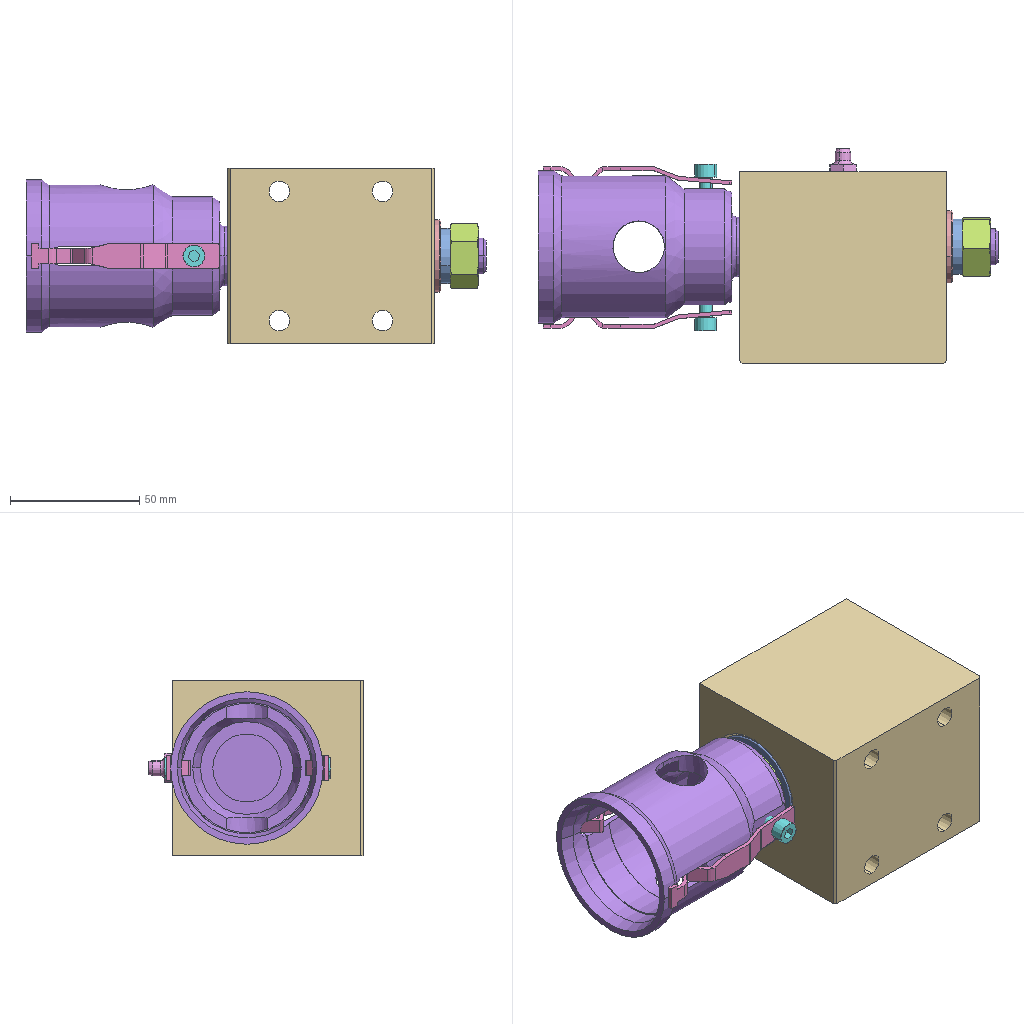Assembly | SolidWorks | 10 different items | 13 placed | box 178 x 83 x 68 mm
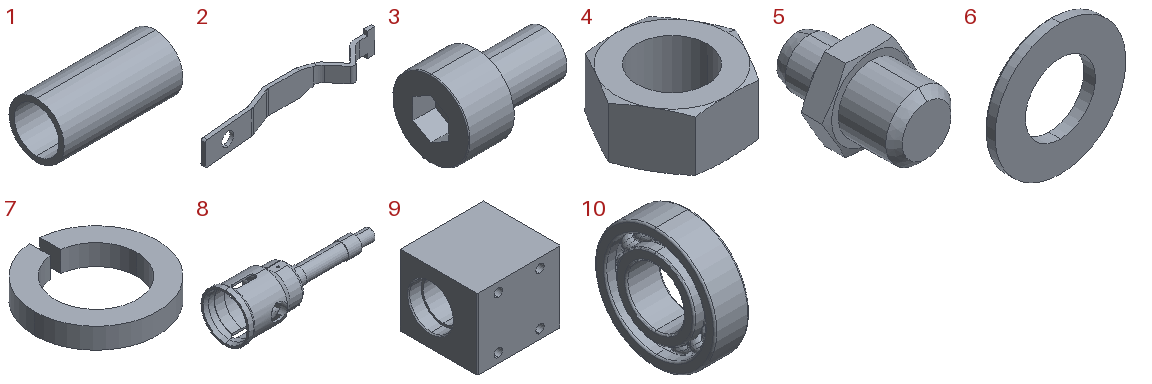Parts list (item | quantity | size | volume | features):
1 | x1 | 56 x 26 x 26 mm | 10336 mm3 | features Extrusion 1
2 | x2 | 73 x 9 x 9.5 mm | 954.396 mm3 | features Extrusion 1, ICE 1
3 | x2 | 13 x 8.5 x 8.5 mm | 404.848 mm3 | features BlendCut 1, Cut 1, Fillet 1, LPattern 1, RevCut 1, Revolution 1
4 | x1 | 25.4 x 21.997 x 11 mm | 2905 mm3 | features Cut 2, Chamfer 1, Extrusion 1
5 | x1 | 11.547 x 15.8 x 10 mm | 760.457 mm3 | features RevCut 2, Chamfer 1, Extrusion 1, ICE 1, Revolution 1
6 | x1 | 28 x 2.5 x 28 mm | 1081 mm3 | features Revolution 1
7 | x1 | 21.361 x 21.323 x 3.6 mm | 696.819 mm3 | features Extrusion 1
8 | x1 | 178 x 59 x 59 mm | 74305 mm3 | features ICE 3, MirrorPattern 1, Revolution 1
9 | x1 | 80 x 74 x 68 mm | 288342 mm3 | features MirrorPattern 3, Chamfer 2, HoleWzd 2, ICE 2, Extrusion 1, MirrorSolid 1
10 | x2 | 12 x 42 x 42 mm | 9401 mm3 | features Revolution 4, CirPattern 2, RefAxis 1, RevCut 1
Mates (type | each side: item.copy, entity, surface, feature):
Concentric | 10.1 face cylinder Revolve1 | 9.1 face cylinder Mirror3
Coincident | 10.1 face plane Revolve1 | 9.1 face plane Mirror2
Coincident | 10.2 face plane Revolve1 | 9.1 face plane Boss-Extrude1
Concentric | 10.2 face cylinder Revolve1 | 9.1 face cylinder Cut-Extrude4
Concentric | 10.1 face cylinder Revolve1 | 8.1 face cylinder Revolve1
Coincident | 10.1 face plane Revolve1 | 8.1 face plane Revolve1
Concentric | 3.1 face cylinder Base-Revolve | 8.1 face cylinder Cut-Extrude1
DistanceDim | 2.1 face plane Boss-Extrude1 | 8.1 face cylinder Revolve1
Parallel | 2.1 face plane Boss-Extrude1 | 8.1 face plane Mirror1
DistanceDim | 3.1 face plane Base-Revolve | 8.1 face plane Mirror1
Concentric | 3.2 face cylinder Base-Revolve | 8.1 face cylinder Cut-Extrude1
DistanceDim | 8.1 face plane Cut-Extrude2 | 3.2 face plane Base-Revolve
Parallel | 2.2 face plane Boss-Extrude1 | 8.1 face plane Cut-Extrude2
DistanceDim | 2.2 face plane Boss-Extrude1 | 8.1 face cylinder Revolve1
Concentric | 2.2 face cylinder Cut-Extrude1 | 3.2 face cylinder Base-Revolve
Concentric | 2.1 face cylinder Cut-Extrude1 | 3.1 face cylinder Base-Revolve
Concentric | 8.1 face cylinder Revolve1 | 1.1 face cylinder Boss-Extrude1
Coincident | 10.1 face plane Revolve1 | 1.1 face plane Boss-Extrude1
Coincident | 9.1 face plane Boss-Extrude1 | 6.1 face plane Base-Revolve
Concentric | 8.1 face cylinder Revolve1 | 6.1 face cylinder Base-Revolve
Concentric | 8.1 face cylinder Revolve1 | 7.1 face cylinder Extrude1
Coincident | 6.1 face plane Base-Revolve | 7.1 face plane Extrude1
Concentric | 8.1 face cylinder Revolve1 | 4.1 face cylinder Base-Extrude
Coincident | 7.1 face plane Extrude1 | 4.1 face plane Base-Extrude
Width | 9.1 face plane Boss-Extrude1 | 9.1 face plane Boss-Extrude1 | 2.1 face plane Boss-Extrude1 | 2.1 face plane Boss-Extrude1
Concentric | 9.1 face cylinder M8 Tapped Hole1 | 5.1 face cylinder Boss-Extrude1
Coincident | 9.1 face plane Boss-Extrude1 | 5.1 face plane Boss-Extrude2